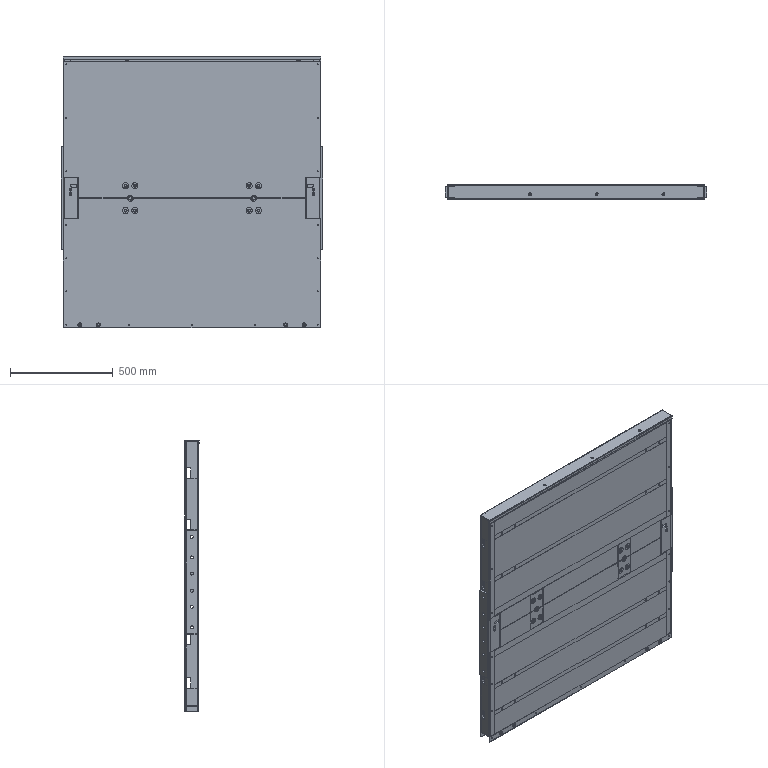Part | 56 solids | 1632 faces | box 1270 x 70 x 1320 mm | volume 12399909 mm3 | plane 984 | cylinder 552 | cone 96 | commonest cylinder face diameters 14.5 x88 10 x78 11 x72 0.4 x36 5 x34 20 x32